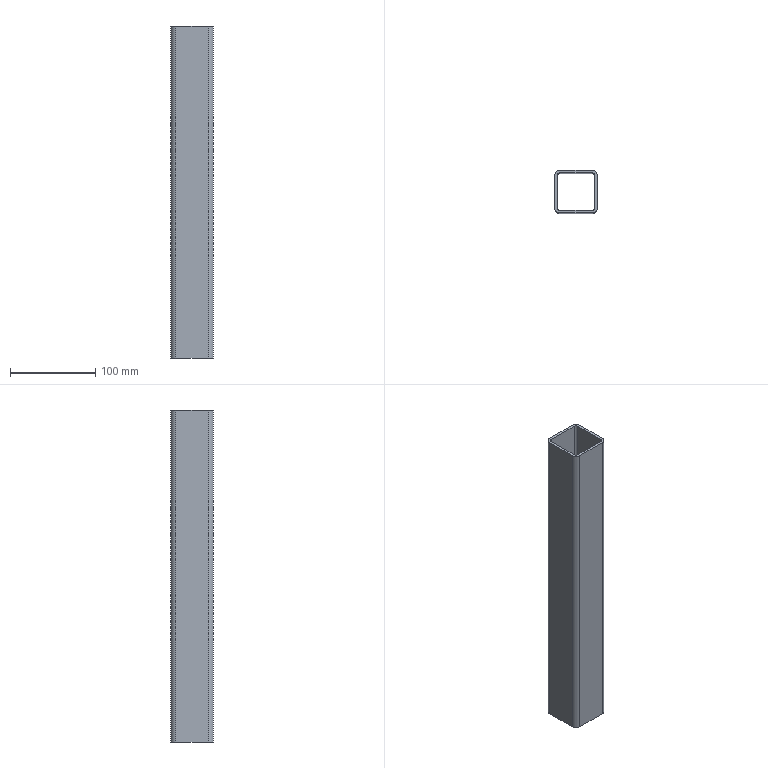Part | SolidWorks | 1 solid | 18 faces | box 50 x 50 x 390 mm | volume 210921 mm3 | plane 10 | cylinder 8 | commonest cylinder face diameters 6 x4 12 x4
STEP:
#1=CARTESIAN_POINT('',(19.,25.,195.));
#2=VERTEX_POINT('',#1);
#3=CARTESIAN_POINT('',(25.,19.,195.));
#4=VERTEX_POINT('',#3);
#5=CARTESIAN_POINT('',(19.,19.,195.));
#6=DIRECTION('',(0.,0.,-1.));
#7=DIRECTION('',(-1.,0.,0.));
#8=AXIS2_PLACEMENT_3D('',#5,#6,#7);
#9=CIRCLE('',#8,6.);
#10=EDGE_CURVE('',#2,#4,#9,.T.);
#11=ORIENTED_EDGE('',*,*,#10,.T.);
#12=CARTESIAN_POINT('',(25.,19.,-195.));
#13=VERTEX_POINT('',#12);
#14=CARTESIAN_POINT('',(25.,19.,-195.));
#15=DIRECTION('',(0.,0.,1.));
#16=VECTOR('',#15,1000.);
#17=LINE('',#14,#16);
#18=EDGE_CURVE('',#13,#4,#17,.T.);
#19=ORIENTED_EDGE('',*,*,#18,.F.);
#20=CARTESIAN_POINT('',(19.,25.,-195.));
#21=VERTEX_POINT('',#20);
#22=CARTESIAN_POINT('',(19.,19.,-195.));
#23=DIRECTION('',(0.,0.,-1.));
#24=DIRECTION('',(-1.,0.,0.));
#25=AXIS2_PLACEMENT_3D('',#22,#23,#24);
#26=CIRCLE('',#25,6.);
#27=EDGE_CURVE('',#21,#13,#26,.T.);
#28=ORIENTED_EDGE('',*,*,#27,.F.);
#29=CARTESIAN_POINT('',(19.,25.,-195.));
#30=DIRECTION('',(0.,0.,1.));
#31=VECTOR('',#30,1000.);
#32=LINE('',#29,#31);
#33=EDGE_CURVE('',#21,#2,#32,.T.);
#34=ORIENTED_EDGE('',*,*,#33,.T.);
#35=EDGE_LOOP('',(#11,#19,#28,#34));
#36=FACE_OUTER_BOUND('',#35,.T.);
#37=CARTESIAN_POINT('',(19.,19.,-195.));
#38=DIRECTION('',(0.,0.,1.));
#39=DIRECTION('',(1.,0.,0.));
#40=AXIS2_PLACEMENT_3D('',#37,#38,#39);
#41=CYLINDRICAL_SURFACE('',#40,6.);
#42=ADVANCED_FACE('',(#36),#41,.T.);
#43=CARTESIAN_POINT('',(25.,-19.,195.));
#44=VERTEX_POINT('',#43);
#45=CARTESIAN_POINT('',(25.,19.,195.));
#46=DIRECTION('',(0.,-1.,0.));
#47=VECTOR('',#46,1000.);
#48=LINE('',#45,#47);
#49=EDGE_CURVE('',#4,#44,#48,.T.);
#50=ORIENTED_EDGE('',*,*,#49,.T.);
#51=CARTESIAN_POINT('',(25.,-19.,-195.));
#52=VERTEX_POINT('',#51);
#53=CARTESIAN_POINT('',(25.,-19.,-195.));
#54=DIRECTION('',(0.,0.,1.));
#55=VECTOR('',#54,1000.);
#56=LINE('',#53,#55);
#57=EDGE_CURVE('',#52,#44,#56,.T.);
#58=ORIENTED_EDGE('',*,*,#57,.F.);
#59=CARTESIAN_POINT('',(25.,19.,-195.));
#60=DIRECTION('',(0.,-1.,0.));
#61=VECTOR('',#60,1000.);
#62=LINE('',#59,#61);
#63=EDGE_CURVE('',#13,#52,#62,.T.);
#64=ORIENTED_EDGE('',*,*,#63,.F.);
#65=ORIENTED_EDGE('',*,*,#18,.T.);
#66=EDGE_LOOP('',(#50,#58,#64,#65));
#67=FACE_OUTER_BOUND('',#66,.T.);
#68=CARTESIAN_POINT('',(25.,19.,-195.));
#69=DIRECTION('',(-1.,0.,0.));
#70=DIRECTION('',(0.,0.,1.));
#71=AXIS2_PLACEMENT_3D('',#68,#69,#70);
#72=PLANE('',#71);
#73=ADVANCED_FACE('',(#67),#72,.F.);
#74=CARTESIAN_POINT('',(19.,-25.,195.));
#75=VERTEX_POINT('',#74);
#76=CARTESIAN_POINT('',(19.,-19.,195.));
#77=DIRECTION('',(0.,0.,-1.));
#78=DIRECTION('',(-1.,0.,0.));
#79=AXIS2_PLACEMENT_3D('',#76,#77,#78);
#80=CIRCLE('',#79,6.);
#81=EDGE_CURVE('',#44,#75,#80,.T.);
#82=ORIENTED_EDGE('',*,*,#81,.T.);
#83=CARTESIAN_POINT('',(19.,-25.,-195.));
#84=VERTEX_POINT('',#83);
#85=CARTESIAN_POINT('',(19.,-25.,-195.));
#86=DIRECTION('',(0.,0.,1.));
#87=VECTOR('',#86,1000.);
#88=LINE('',#85,#87);
#89=EDGE_CURVE('',#84,#75,#88,.T.);
#90=ORIENTED_EDGE('',*,*,#89,.F.);
#91=CARTESIAN_POINT('',(19.,-19.,-195.));
#92=DIRECTION('',(0.,0.,-1.));
#93=DIRECTION('',(-1.,0.,0.));
#94=AXIS2_PLACEMENT_3D('',#91,#92,#93);
#95=CIRCLE('',#94,6.);
#96=EDGE_CURVE('',#52,#84,#95,.T.);
#97=ORIENTED_EDGE('',*,*,#96,.F.);
#98=ORIENTED_EDGE('',*,*,#57,.T.);
#99=EDGE_LOOP('',(#82,#90,#97,#98));
#100=FACE_OUTER_BOUND('',#99,.T.);
#101=CARTESIAN_POINT('',(19.,-19.,-195.));
#102=DIRECTION('',(0.,0.,1.));
#103=DIRECTION('',(1.,0.,0.));
#104=AXIS2_PLACEMENT_3D('',#101,#102,#103);
#105=CYLINDRICAL_SURFACE('',#104,6.);
#106=ADVANCED_FACE('',(#100),#105,.T.);
#107=CARTESIAN_POINT('',(-19.,-25.,195.));
#108=VERTEX_POINT('',#107);
#109=CARTESIAN_POINT('',(-19.,-25.,195.));
#110=DIRECTION('',(-1.,0.,0.));
#111=VECTOR('',#110,1000.);
#112=LINE('',#109,#111);
#113=EDGE_CURVE('',#75,#108,#112,.T.);
#114=ORIENTED_EDGE('',*,*,#113,.T.);
#115=CARTESIAN_POINT('',(-19.,-25.,-195.));
#116=VERTEX_POINT('',#115);
#117=CARTESIAN_POINT('',(-19.,-25.,-195.));
#118=DIRECTION('',(0.,0.,1.));
#119=VECTOR('',#118,1000.);
#120=LINE('',#117,#119);
#121=EDGE_CURVE('',#116,#108,#120,.T.);
#122=ORIENTED_EDGE('',*,*,#121,.F.);
#123=CARTESIAN_POINT('',(-19.,-25.,-195.));
#124=DIRECTION('',(-1.,0.,0.));
#125=VECTOR('',#124,1000.);
#126=LINE('',#123,#125);
#127=EDGE_CURVE('',#84,#116,#126,.T.);
#128=ORIENTED_EDGE('',*,*,#127,.F.);
#129=ORIENTED_EDGE('',*,*,#89,.T.);
#130=EDGE_LOOP('',(#114,#122,#128,#129));
#131=FACE_OUTER_BOUND('',#130,.T.);
#132=CARTESIAN_POINT('',(-19.,-25.,-195.));
#133=DIRECTION('',(0.,1.,0.));
#134=DIRECTION('',(0.,0.,1.));
#135=AXIS2_PLACEMENT_3D('',#132,#133,#134);
#136=PLANE('',#135);
#137=ADVANCED_FACE('',(#131),#136,.F.);
#138=CARTESIAN_POINT('',(-25.,-19.,195.));
#139=VERTEX_POINT('',#138);
#140=CARTESIAN_POINT('',(-19.,-19.,195.));
#141=DIRECTION('',(0.,0.,-1.));
#142=DIRECTION('',(-1.,0.,0.));
#143=AXIS2_PLACEMENT_3D('',#140,#141,#142);
#144=CIRCLE('',#143,6.);
#145=EDGE_CURVE('',#108,#139,#144,.T.);
#146=ORIENTED_EDGE('',*,*,#145,.T.);
#147=CARTESIAN_POINT('',(-25.,-19.,-195.));
#148=VERTEX_POINT('',#147);
#149=CARTESIAN_POINT('',(-25.,-19.,-195.));
#150=DIRECTION('',(0.,0.,1.));
#151=VECTOR('',#150,1000.);
#152=LINE('',#149,#151);
#153=EDGE_CURVE('',#148,#139,#152,.T.);
#154=ORIENTED_EDGE('',*,*,#153,.F.);
#155=CARTESIAN_POINT('',(-19.,-19.,-195.));
#156=DIRECTION('',(0.,0.,-1.));
#157=DIRECTION('',(-1.,0.,0.));
#158=AXIS2_PLACEMENT_3D('',#155,#156,#157);
#159=CIRCLE('',#158,6.);
#160=EDGE_CURVE('',#116,#148,#159,.T.);
#161=ORIENTED_EDGE('',*,*,#160,.F.);
#162=ORIENTED_EDGE('',*,*,#121,.T.);
#163=EDGE_LOOP('',(#146,#154,#161,#162));
#164=FACE_OUTER_BOUND('',#163,.T.);
#165=CARTESIAN_POINT('',(-19.,-19.,-195.));
#166=DIRECTION('',(0.,0.,1.));
#167=DIRECTION('',(1.,0.,0.));
#168=AXIS2_PLACEMENT_3D('',#165,#166,#167);
#169=CYLINDRICAL_SURFACE('',#168,6.);
#170=ADVANCED_FACE('',(#164),#169,.T.);
#171=CARTESIAN_POINT('',(-25.,19.,195.));
#172=VERTEX_POINT('',#171);
#173=CARTESIAN_POINT('',(-25.,-19.,195.));
#174=DIRECTION('',(0.,1.,0.));
#175=VECTOR('',#174,1000.);
#176=LINE('',#173,#175);
#177=EDGE_CURVE('',#139,#172,#176,.T.);
#178=ORIENTED_EDGE('',*,*,#177,.T.);
#179=CARTESIAN_POINT('',(-25.,19.,-195.));
#180=VERTEX_POINT('',#179);
#181=CARTESIAN_POINT('',(-25.,19.,-195.));
#182=DIRECTION('',(0.,0.,1.));
#183=VECTOR('',#182,1000.);
#184=LINE('',#181,#183);
#185=EDGE_CURVE('',#180,#172,#184,.T.);
#186=ORIENTED_EDGE('',*,*,#185,.F.);
#187=CARTESIAN_POINT('',(-25.,-19.,-195.));
#188=DIRECTION('',(0.,1.,0.));
#189=VECTOR('',#188,1000.);
#190=LINE('',#187,#189);
#191=EDGE_CURVE('',#148,#180,#190,.T.);
#192=ORIENTED_EDGE('',*,*,#191,.F.);
#193=ORIENTED_EDGE('',*,*,#153,.T.);
#194=EDGE_LOOP('',(#178,#186,#192,#193));
#195=FACE_OUTER_BOUND('',#194,.T.);
#196=CARTESIAN_POINT('',(-25.,-19.,-195.));
#197=DIRECTION('',(1.,0.,0.));
#198=DIRECTION('',(0.,0.,-1.));
#199=AXIS2_PLACEMENT_3D('',#196,#197,#198);
#200=PLANE('',#199);
#201=ADVANCED_FACE('',(#195),#200,.F.);
#202=CARTESIAN_POINT('',(-19.,25.,195.));
#203=VERTEX_POINT('',#202);
#204=CARTESIAN_POINT('',(-19.,19.,195.));
#205=DIRECTION('',(0.,0.,-1.));
#206=DIRECTION('',(-1.,0.,0.));
#207=AXIS2_PLACEMENT_3D('',#204,#205,#206);
#208=CIRCLE('',#207,6.);
#209=EDGE_CURVE('',#172,#203,#208,.T.);
#210=ORIENTED_EDGE('',*,*,#209,.T.);
#211=CARTESIAN_POINT('',(-19.,25.,-195.));
#212=VERTEX_POINT('',#211);
#213=CARTESIAN_POINT('',(-19.,25.,-195.));
#214=DIRECTION('',(0.,0.,1.));
#215=VECTOR('',#214,1000.);
#216=LINE('',#213,#215);
#217=EDGE_CURVE('',#212,#203,#216,.T.);
#218=ORIENTED_EDGE('',*,*,#217,.F.);
#219=CARTESIAN_POINT('',(-19.,19.,-195.));
#220=DIRECTION('',(0.,0.,-1.));
#221=DIRECTION('',(-1.,0.,0.));
#222=AXIS2_PLACEMENT_3D('',#219,#220,#221);
#223=CIRCLE('',#222,6.);
#224=EDGE_CURVE('',#180,#212,#223,.T.);
#225=ORIENTED_EDGE('',*,*,#224,.F.);
#226=ORIENTED_EDGE('',*,*,#185,.T.);
#227=EDGE_LOOP('',(#210,#218,#225,#226));
#228=FACE_OUTER_BOUND('',#227,.T.);
#229=CARTESIAN_POINT('',(-19.,19.,-195.));
#230=DIRECTION('',(0.,0.,1.));
#231=DIRECTION('',(1.,0.,0.));
#232=AXIS2_PLACEMENT_3D('',#229,#230,#231);
#233=CYLINDRICAL_SURFACE('',#232,6.);
#234=ADVANCED_FACE('',(#228),#233,.T.);
#235=CARTESIAN_POINT('',(22.,-19.,195.));
#236=VERTEX_POINT('',#235);
#237=CARTESIAN_POINT('',(19.,-22.,195.));
#238=VERTEX_POINT('',#237);
#239=CARTESIAN_POINT('',(19.,-19.,195.));
#240=DIRECTION('',(0.,0.,-1.));
#241=DIRECTION('',(-1.,0.,0.));
#242=AXIS2_PLACEMENT_3D('',#239,#240,#241);
#243=CIRCLE('',#242,3.);
#244=EDGE_CURVE('',#236,#238,#243,.T.);
#245=ORIENTED_EDGE('',*,*,#244,.F.);
#246=CARTESIAN_POINT('',(22.,-19.,-195.));
#247=VERTEX_POINT('',#246);
#248=CARTESIAN_POINT('',(22.,-19.,-195.));
#249=DIRECTION('',(0.,0.,1.));
#250=VECTOR('',#249,1000.);
#251=LINE('',#248,#250);
#252=EDGE_CURVE('',#247,#236,#251,.T.);
#253=ORIENTED_EDGE('',*,*,#252,.F.);
#254=CARTESIAN_POINT('',(19.,-22.,-195.));
#255=VERTEX_POINT('',#254);
#256=CARTESIAN_POINT('',(19.,-19.,-195.));
#257=DIRECTION('',(0.,0.,-1.));
#258=DIRECTION('',(-1.,0.,0.));
#259=AXIS2_PLACEMENT_3D('',#256,#257,#258);
#260=CIRCLE('',#259,3.);
#261=EDGE_CURVE('',#247,#255,#260,.T.);
#262=ORIENTED_EDGE('',*,*,#261,.T.);
#263=CARTESIAN_POINT('',(19.,-22.,-195.));
#264=DIRECTION('',(0.,0.,1.));
#265=VECTOR('',#264,1000.);
#266=LINE('',#263,#265);
#267=EDGE_CURVE('',#255,#238,#266,.T.);
#268=ORIENTED_EDGE('',*,*,#267,.T.);
#269=EDGE_LOOP('',(#245,#253,#262,#268));
#270=FACE_OUTER_BOUND('',#269,.T.);
#271=CARTESIAN_POINT('',(19.,-19.,-195.));
#272=DIRECTION('',(0.,0.,1.));
#273=DIRECTION('',(1.,0.,0.));
#274=AXIS2_PLACEMENT_3D('',#271,#272,#273);
#275=CYLINDRICAL_SURFACE('',#274,3.);
#276=ADVANCED_FACE('',(#270),#275,.F.);
#277=CARTESIAN_POINT('',(22.,19.,195.));
#278=VERTEX_POINT('',#277);
#279=CARTESIAN_POINT('',(22.,19.,195.));
#280=DIRECTION('',(0.,-1.,0.));
#281=VECTOR('',#280,1000.);
#282=LINE('',#279,#281);
#283=EDGE_CURVE('',#278,#236,#282,.T.);
#284=ORIENTED_EDGE('',*,*,#283,.F.);
#285=CARTESIAN_POINT('',(22.,19.,-195.));
#286=VERTEX_POINT('',#285);
#287=CARTESIAN_POINT('',(22.,19.,-195.));
#288=DIRECTION('',(0.,0.,1.));
#289=VECTOR('',#288,1000.);
#290=LINE('',#287,#289);
#291=EDGE_CURVE('',#286,#278,#290,.T.);
#292=ORIENTED_EDGE('',*,*,#291,.F.);
#293=CARTESIAN_POINT('',(22.,19.,-195.));
#294=DIRECTION('',(0.,-1.,0.));
#295=VECTOR('',#294,1000.);
#296=LINE('',#293,#295);
#297=EDGE_CURVE('',#286,#247,#296,.T.);
#298=ORIENTED_EDGE('',*,*,#297,.T.);
#299=ORIENTED_EDGE('',*,*,#252,.T.);
#300=EDGE_LOOP('',(#284,#292,#298,#299));
#301=FACE_OUTER_BOUND('',#300,.T.);
#302=CARTESIAN_POINT('',(22.,19.,-195.));
#303=DIRECTION('',(-1.,0.,0.));
#304=DIRECTION('',(0.,0.,1.));
#305=AXIS2_PLACEMENT_3D('',#302,#303,#304);
#306=PLANE('',#305);
#307=ADVANCED_FACE('',(#301),#306,.T.);
#308=CARTESIAN_POINT('',(19.,22.,195.));
#309=VERTEX_POINT('',#308);
#310=CARTESIAN_POINT('',(19.,19.,195.));
#311=DIRECTION('',(0.,0.,-1.));
#312=DIRECTION('',(-1.,0.,0.));
#313=AXIS2_PLACEMENT_3D('',#310,#311,#312);
#314=CIRCLE('',#313,3.);
#315=EDGE_CURVE('',#309,#278,#314,.T.);
#316=ORIENTED_EDGE('',*,*,#315,.F.);
#317=CARTESIAN_POINT('',(19.,22.,-195.));
#318=VERTEX_POINT('',#317);
#319=CARTESIAN_POINT('',(19.,22.,-195.));
#320=DIRECTION('',(0.,0.,1.));
#321=VECTOR('',#320,1000.);
#322=LINE('',#319,#321);
#323=EDGE_CURVE('',#318,#309,#322,.T.);
#324=ORIENTED_EDGE('',*,*,#323,.F.);
#325=CARTESIAN_POINT('',(19.,19.,-195.));
#326=DIRECTION('',(0.,0.,-1.));
#327=DIRECTION('',(-1.,0.,0.));
#328=AXIS2_PLACEMENT_3D('',#325,#326,#327);
#329=CIRCLE('',#328,3.);
#330=EDGE_CURVE('',#318,#286,#329,.T.);
#331=ORIENTED_EDGE('',*,*,#330,.T.);
#332=ORIENTED_EDGE('',*,*,#291,.T.);
#333=EDGE_LOOP('',(#316,#324,#331,#332));
#334=FACE_OUTER_BOUND('',#333,.T.);
#335=CARTESIAN_POINT('',(19.,19.,-195.));
#336=DIRECTION('',(0.,0.,1.));
#337=DIRECTION('',(1.,0.,0.));
#338=AXIS2_PLACEMENT_3D('',#335,#336,#337);
#339=CYLINDRICAL_SURFACE('',#338,3.);
#340=ADVANCED_FACE('',(#334),#339,.F.);
#341=CARTESIAN_POINT('',(-19.,22.,195.));
#342=VERTEX_POINT('',#341);
#343=CARTESIAN_POINT('',(19.,22.,195.));
#344=DIRECTION('',(1.,0.,0.));
#345=VECTOR('',#344,1000.);
#346=LINE('',#343,#345);
#347=EDGE_CURVE('',#342,#309,#346,.T.);
#348=ORIENTED_EDGE('',*,*,#347,.F.);
#349=CARTESIAN_POINT('',(-19.,22.,-195.));
#350=VERTEX_POINT('',#349);
#351=CARTESIAN_POINT('',(-19.,22.,-195.));
#352=DIRECTION('',(0.,0.,1.));
#353=VECTOR('',#352,1000.);
#354=LINE('',#351,#353);
#355=EDGE_CURVE('',#350,#342,#354,.T.);
#356=ORIENTED_EDGE('',*,*,#355,.F.);
#357=CARTESIAN_POINT('',(19.,22.,-195.));
#358=DIRECTION('',(1.,0.,0.));
#359=VECTOR('',#358,1000.);
#360=LINE('',#357,#359);
#361=EDGE_CURVE('',#350,#318,#360,.T.);
#362=ORIENTED_EDGE('',*,*,#361,.T.);
#363=ORIENTED_EDGE('',*,*,#323,.T.);
#364=EDGE_LOOP('',(#348,#356,#362,#363));
#365=FACE_OUTER_BOUND('',#364,.T.);
#366=CARTESIAN_POINT('',(19.,22.,-195.));
#367=DIRECTION('',(0.,-1.,0.));
#368=DIRECTION('',(0.,0.,-1.));
#369=AXIS2_PLACEMENT_3D('',#366,#367,#368);
#370=PLANE('',#369);
#371=ADVANCED_FACE('',(#365),#370,.T.);
#372=CARTESIAN_POINT('',(-22.,19.,195.));
#373=VERTEX_POINT('',#372);
#374=CARTESIAN_POINT('',(-19.,19.,195.));
#375=DIRECTION('',(0.,0.,-1.));
#376=DIRECTION('',(-1.,0.,0.));
#377=AXIS2_PLACEMENT_3D('',#374,#375,#376);
#378=CIRCLE('',#377,3.);
#379=EDGE_CURVE('',#373,#342,#378,.T.);
#380=ORIENTED_EDGE('',*,*,#379,.F.);
#381=CARTESIAN_POINT('',(-22.,19.,-195.));
#382=VERTEX_POINT('',#381);
#383=CARTESIAN_POINT('',(-22.,19.,-195.));
#384=DIRECTION('',(0.,0.,1.));
#385=VECTOR('',#384,1000.);
#386=LINE('',#383,#385);
#387=EDGE_CURVE('',#382,#373,#386,.T.);
#388=ORIENTED_EDGE('',*,*,#387,.F.);
#389=CARTESIAN_POINT('',(-19.,19.,-195.));
#390=DIRECTION('',(0.,0.,-1.));
#391=DIRECTION('',(-1.,0.,0.));
#392=AXIS2_PLACEMENT_3D('',#389,#390,#391);
#393=CIRCLE('',#392,3.);
#394=EDGE_CURVE('',#382,#350,#393,.T.);
#395=ORIENTED_EDGE('',*,*,#394,.T.);
#396=ORIENTED_EDGE('',*,*,#355,.T.);
#397=EDGE_LOOP('',(#380,#388,#395,#396));
#398=FACE_OUTER_BOUND('',#397,.T.);
#399=CARTESIAN_POINT('',(-19.,19.,-195.));
#400=DIRECTION('',(0.,0.,1.));
#401=DIRECTION('',(1.,0.,0.));
#402=AXIS2_PLACEMENT_3D('',#399,#400,#401);
#403=CYLINDRICAL_SURFACE('',#402,3.);
#404=ADVANCED_FACE('',(#398),#403,.F.);
#405=CARTESIAN_POINT('',(-22.,-19.,195.));
#406=VERTEX_POINT('',#405);
#407=CARTESIAN_POINT('',(-22.,-19.,195.));
#408=DIRECTION('',(0.,1.,0.));
#409=VECTOR('',#408,1000.);
#410=LINE('',#407,#409);
#411=EDGE_CURVE('',#406,#373,#410,.T.);
#412=ORIENTED_EDGE('',*,*,#411,.F.);
#413=CARTESIAN_POINT('',(-22.,-19.,-195.));
#414=VERTEX_POINT('',#413);
#415=CARTESIAN_POINT('',(-22.,-19.,-195.));
#416=DIRECTION('',(0.,0.,1.));
#417=VECTOR('',#416,1000.);
#418=LINE('',#415,#417);
#419=EDGE_CURVE('',#414,#406,#418,.T.);
#420=ORIENTED_EDGE('',*,*,#419,.F.);
#421=CARTESIAN_POINT('',(-22.,-19.,-195.));
#422=DIRECTION('',(0.,1.,0.));
#423=VECTOR('',#422,1000.);
#424=LINE('',#421,#423);
#425=EDGE_CURVE('',#414,#382,#424,.T.);
#426=ORIENTED_EDGE('',*,*,#425,.T.);
#427=ORIENTED_EDGE('',*,*,#387,.T.);
#428=EDGE_LOOP('',(#412,#420,#426,#427));
#429=FACE_OUTER_BOUND('',#428,.T.);
#430=CARTESIAN_POINT('',(-22.,-19.,-195.));
#431=DIRECTION('',(1.,0.,0.));
#432=DIRECTION('',(0.,0.,-1.));
#433=AXIS2_PLACEMENT_3D('',#430,#431,#432);
#434=PLANE('',#433);
#435=ADVANCED_FACE('',(#429),#434,.T.);
#436=CARTESIAN_POINT('',(-19.,-22.,195.));
#437=VERTEX_POINT('',#436);
#438=CARTESIAN_POINT('',(-19.,-19.,195.));
#439=DIRECTION('',(0.,0.,-1.));
#440=DIRECTION('',(-1.,0.,0.));
#441=AXIS2_PLACEMENT_3D('',#438,#439,#440);
#442=CIRCLE('',#441,3.);
#443=EDGE_CURVE('',#437,#406,#442,.T.);
#444=ORIENTED_EDGE('',*,*,#443,.F.);
#445=CARTESIAN_POINT('',(-19.,-22.,-195.));
#446=VERTEX_POINT('',#445);
#447=CARTESIAN_POINT('',(-19.,-22.,-195.));
#448=DIRECTION('',(0.,0.,1.));
#449=VECTOR('',#448,1000.);
#450=LINE('',#447,#449);
#451=EDGE_CURVE('',#446,#437,#450,.T.);
#452=ORIENTED_EDGE('',*,*,#451,.F.);
#453=CARTESIAN_POINT('',(-19.,-19.,-195.));
#454=DIRECTION('',(0.,0.,-1.));
#455=DIRECTION('',(-1.,0.,0.));
#456=AXIS2_PLACEMENT_3D('',#453,#454,#455);
#457=CIRCLE('',#456,3.);
#458=EDGE_CURVE('',#446,#414,#457,.T.);
#459=ORIENTED_EDGE('',*,*,#458,.T.);
#460=ORIENTED_EDGE('',*,*,#419,.T.);
#461=EDGE_LOOP('',(#444,#452,#459,#460));
#462=FACE_OUTER_BOUND('',#461,.T.);
#463=CARTESIAN_POINT('',(-19.,-19.,-195.));
#464=DIRECTION('',(0.,0.,1.));
#465=DIRECTION('',(1.,0.,0.));
#466=AXIS2_PLACEMENT_3D('',#463,#464,#465);
#467=CYLINDRICAL_SURFACE('',#466,3.);
#468=ADVANCED_FACE('',(#462),#467,.F.);
#469=CARTESIAN_POINT('',(-19.,-22.,195.));
#470=DIRECTION('',(-1.,0.,0.));
#471=VECTOR('',#470,1000.);
#472=LINE('',#469,#471);
#473=EDGE_CURVE('',#238,#437,#472,.T.);
#474=ORIENTED_EDGE('',*,*,#473,.F.);
#475=ORIENTED_EDGE('',*,*,#267,.F.);
#476=CARTESIAN_POINT('',(-19.,-22.,-195.));
#477=DIRECTION('',(-1.,0.,0.));
#478=VECTOR('',#477,1000.);
#479=LINE('',#476,#478);
#480=EDGE_CURVE('',#255,#446,#479,.T.);
#481=ORIENTED_EDGE('',*,*,#480,.T.);
#482=ORIENTED_EDGE('',*,*,#451,.T.);
#483=EDGE_LOOP('',(#474,#475,#481,#482));
#484=FACE_OUTER_BOUND('',#483,.T.);
#485=CARTESIAN_POINT('',(-19.,-22.,-195.));
#486=DIRECTION('',(0.,1.,0.));
#487=DIRECTION('',(0.,0.,1.));
#488=AXIS2_PLACEMENT_3D('',#485,#486,#487);
#489=PLANE('',#488);
#490=ADVANCED_FACE('',(#484),#489,.T.);
#491=CARTESIAN_POINT('',(19.,25.,195.));
#492=DIRECTION('',(1.,0.,0.));
#493=VECTOR('',#492,1000.);
#494=LINE('',#491,#493);
#495=EDGE_CURVE('',#203,#2,#494,.T.);
#496=ORIENTED_EDGE('',*,*,#495,.T.);
#497=ORIENTED_EDGE('',*,*,#33,.F.);
#498=CARTESIAN_POINT('',(19.,25.,-195.));
#499=DIRECTION('',(1.,0.,0.));
#500=VECTOR('',#499,1000.);
#501=LINE('',#498,#500);
#502=EDGE_CURVE('',#212,#21,#501,.T.);
#503=ORIENTED_EDGE('',*,*,#502,.F.);
#504=ORIENTED_EDGE('',*,*,#217,.T.);
#505=EDGE_LOOP('',(#496,#497,#503,#504));
#506=FACE_OUTER_BOUND('',#505,.T.);
#507=CARTESIAN_POINT('',(19.,25.,-195.));
#508=DIRECTION('',(0.,-1.,0.));
#509=DIRECTION('',(0.,0.,-1.));
#510=AXIS2_PLACEMENT_3D('',#507,#508,#509);
#511=PLANE('',#510);
#512=ADVANCED_FACE('',(#506),#511,.F.);
#513=ORIENTED_EDGE('',*,*,#261,.F.);
#514=ORIENTED_EDGE('',*,*,#297,.F.);
#515=ORIENTED_EDGE('',*,*,#330,.F.);
#516=ORIENTED_EDGE('',*,*,#361,.F.);
#517=ORIENTED_EDGE('',*,*,#394,.F.);
#518=ORIENTED_EDGE('',*,*,#425,.F.);
#519=ORIENTED_EDGE('',*,*,#458,.F.);
#520=ORIENTED_EDGE('',*,*,#480,.F.);
#521=EDGE_LOOP('',(#513,#514,#515,#516,#517,#518,#519,#520));
#522=FACE_BOUND('',#521,.T.);
#523=ORIENTED_EDGE('',*,*,#27,.T.);
#524=ORIENTED_EDGE('',*,*,#63,.T.);
#525=ORIENTED_EDGE('',*,*,#96,.T.);
#526=ORIENTED_EDGE('',*,*,#127,.T.);
#527=ORIENTED_EDGE('',*,*,#160,.T.);
#528=ORIENTED_EDGE('',*,*,#191,.T.);
#529=ORIENTED_EDGE('',*,*,#224,.T.);
#530=ORIENTED_EDGE('',*,*,#502,.T.);
#531=EDGE_LOOP('',(#523,#524,#525,#526,#527,#528,#529,#530));
#532=FACE_OUTER_BOUND('',#531,.T.);
#533=CARTESIAN_POINT('',(19.,19.,-195.));
#534=DIRECTION('',(0.,0.,-1.));
#535=DIRECTION('',(-1.,0.,0.));
#536=AXIS2_PLACEMENT_3D('',#533,#534,#535);
#537=PLANE('',#536);
#538=ADVANCED_FACE('',(#522,#532),#537,.T.);
#539=ORIENTED_EDGE('',*,*,#244,.T.);
#540=ORIENTED_EDGE('',*,*,#473,.T.);
#541=ORIENTED_EDGE('',*,*,#443,.T.);
#542=ORIENTED_EDGE('',*,*,#411,.T.);
#543=ORIENTED_EDGE('',*,*,#379,.T.);
#544=ORIENTED_EDGE('',*,*,#347,.T.);
#545=ORIENTED_EDGE('',*,*,#315,.T.);
#546=ORIENTED_EDGE('',*,*,#283,.T.);
#547=EDGE_LOOP('',(#539,#540,#541,#542,#543,#544,#545,#546));
#548=FACE_BOUND('',#547,.T.);
#549=ORIENTED_EDGE('',*,*,#10,.F.);
#550=ORIENTED_EDGE('',*,*,#495,.F.);
#551=ORIENTED_EDGE('',*,*,#209,.F.);
#552=ORIENTED_EDGE('',*,*,#177,.F.);
#553=ORIENTED_EDGE('',*,*,#145,.F.);
#554=ORIENTED_EDGE('',*,*,#113,.F.);
#555=ORIENTED_EDGE('',*,*,#81,.F.);
#556=ORIENTED_EDGE('',*,*,#49,.F.);
#557=EDGE_LOOP('',(#549,#550,#551,#552,#553,#554,#555,#556));
#558=FACE_OUTER_BOUND('',#557,.T.);
#559=CARTESIAN_POINT('',(19.,19.,195.));
#560=DIRECTION('',(0.,0.,-1.));
#561=DIRECTION('',(-1.,0.,0.));
#562=AXIS2_PLACEMENT_3D('',#559,#560,#561);
#563=PLANE('',#562);
#564=ADVANCED_FACE('',(#548,#558),#563,.F.);
#565=CLOSED_SHELL('',(#42,#73,#106,#137,#170,#201,#234,#276,#307,#340,#371,#404,#435,#468,#490,#512,#538,#564));
#566=MANIFOLD_SOLID_BREP('',#565);
#567=CARTESIAN_POINT('',(0.,0.,0.));
#568=DIRECTION('',(0.,0.,1.));
#569=DIRECTION('',(1.,0.,0.));
#570=AXIS2_PLACEMENT_3D('',#567,#568,#569);
#571=(LENGTH_UNIT()NAMED_UNIT(*)SI_UNIT(.MILLI.,.METRE.));
#572=UNCERTAINTY_MEASURE_WITH_UNIT(LENGTH_MEASURE(0.00001),#571,'','');
#573=(NAMED_UNIT(*)PLANE_ANGLE_UNIT()SI_UNIT($,.RADIAN.));
#574=(NAMED_UNIT(*)SI_UNIT($,.STERADIAN.)SOLID_ANGLE_UNIT());
#575=(GEOMETRIC_REPRESENTATION_CONTEXT(3)GLOBAL_UNCERTAINTY_ASSIGNED_CONTEXT((#572))GLOBAL_UNIT_ASSIGNED_CONTEXT((#571,#573,#574))REPRESENTATION_CONTEXT('',''));
#576=ADVANCED_BREP_SHAPE_REPRESENTATION('',(#566,#570),#575);